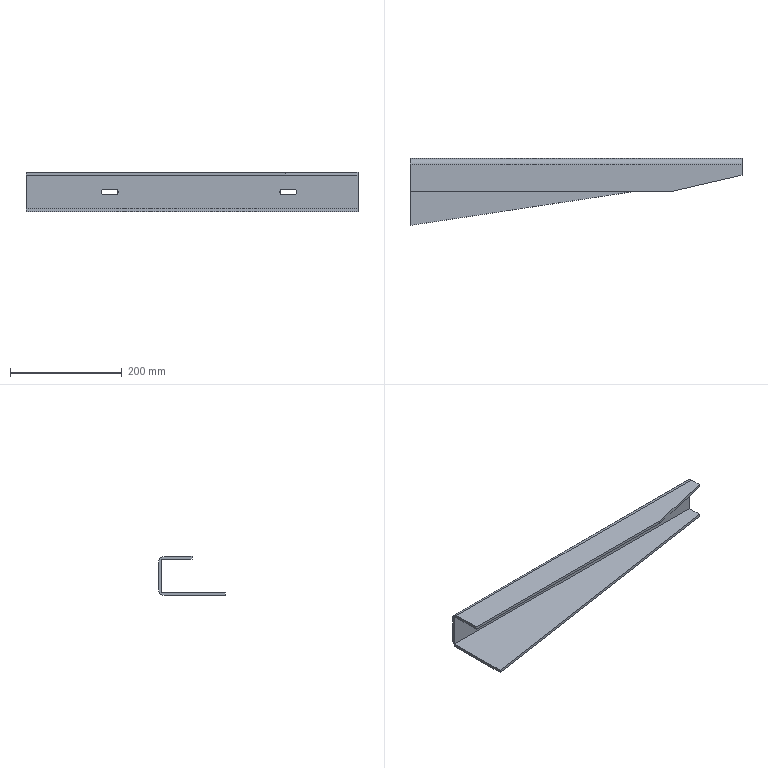Part | SolidWorks | features ICE 3, Fillet 2, Extrusion 1, Shell 1 | 1 solid | 21 faces | box 595 x 120 x 70 mm | volume 542052 mm3 | plane 15 | cylinder 6 | commonest cylinder face diameters 10 x4 20 x2
STEP:
#1=CARTESIAN_POINT('',(160.,70.,40.));
#2=VERTEX_POINT('',#1);
#3=CARTESIAN_POINT('',(140.,70.,40.));
#4=VERTEX_POINT('',#3);
#5=CARTESIAN_POINT('',(0.,70.,40.));
#6=DIRECTION('',(-1.,0.,0.));
#7=VECTOR('',#6,1000.);
#8=LINE('',#5,#7);
#9=EDGE_CURVE('',#2,#4,#8,.T.);
#10=ORIENTED_EDGE('',*,*,#9,.T.);
#11=CARTESIAN_POINT('',(140.,70.,30.));
#12=VERTEX_POINT('',#11);
#13=CARTESIAN_POINT('',(140.,70.,35.));
#14=DIRECTION('',(0.,1.,0.));
#15=DIRECTION('',(0.,0.,1.));
#16=AXIS2_PLACEMENT_3D('',#13,#14,#15);
#17=CIRCLE('',#16,5.);
#18=EDGE_CURVE('',#12,#4,#17,.T.);
#19=ORIENTED_EDGE('',*,*,#18,.F.);
#20=CARTESIAN_POINT('',(160.,70.,30.));
#21=VERTEX_POINT('',#20);
#22=CARTESIAN_POINT('',(0.,70.,30.));
#23=DIRECTION('',(1.,0.,0.));
#24=VECTOR('',#23,1000.);
#25=LINE('',#22,#24);
#26=EDGE_CURVE('',#12,#21,#25,.T.);
#27=ORIENTED_EDGE('',*,*,#26,.T.);
#28=CARTESIAN_POINT('',(160.,70.,35.));
#29=DIRECTION('',(0.,1.,0.));
#30=DIRECTION('',(0.,0.,1.));
#31=AXIS2_PLACEMENT_3D('',#28,#29,#30);
#32=CIRCLE('',#31,5.);
#33=EDGE_CURVE('',#2,#21,#32,.T.);
#34=ORIENTED_EDGE('',*,*,#33,.F.);
#35=EDGE_LOOP('',(#10,#19,#27,#34));
#36=FACE_BOUND('',#35,.T.);
#37=CARTESIAN_POINT('',(595.,70.,60.));
#38=VERTEX_POINT('',#37);
#39=CARTESIAN_POINT('',(595.,70.,10.));
#40=VERTEX_POINT('',#39);
#41=CARTESIAN_POINT('',(595.,70.,70.));
#42=DIRECTION('',(0.,0.,-1.));
#43=VECTOR('',#42,1000.);
#44=LINE('',#41,#43);
#45=EDGE_CURVE('',#38,#40,#44,.T.);
#46=ORIENTED_EDGE('',*,*,#45,.T.);
#47=CARTESIAN_POINT('',(0.,70.,10.));
#48=VERTEX_POINT('',#47);
#49=CARTESIAN_POINT('',(0.,70.,10.));
#50=DIRECTION('',(-1.,0.,0.));
#51=VECTOR('',#50,1000.);
#52=LINE('',#49,#51);
#53=EDGE_CURVE('',#40,#48,#52,.T.);
#54=ORIENTED_EDGE('',*,*,#53,.T.);
#55=CARTESIAN_POINT('',(0.,70.,60.));
#56=VERTEX_POINT('',#55);
#57=CARTESIAN_POINT('',(0.,70.,70.));
#58=DIRECTION('',(0.,0.,-1.));
#59=VECTOR('',#58,1000.);
#60=LINE('',#57,#59);
#61=EDGE_CURVE('',#56,#48,#60,.T.);
#62=ORIENTED_EDGE('',*,*,#61,.F.);
#63=CARTESIAN_POINT('',(570.,70.,60.));
#64=DIRECTION('',(1.,0.,0.));
#65=VECTOR('',#64,1000.);
#66=LINE('',#63,#65);
#67=EDGE_CURVE('',#56,#38,#66,.T.);
#68=ORIENTED_EDGE('',*,*,#67,.T.);
#69=EDGE_LOOP('',(#46,#54,#62,#68));
#70=FACE_OUTER_BOUND('',#69,.T.);
#71=CARTESIAN_POINT('',(460.,70.,30.));
#72=VERTEX_POINT('',#71);
#73=CARTESIAN_POINT('',(480.,70.,30.));
#74=VERTEX_POINT('',#73);
#75=CARTESIAN_POINT('',(0.,70.,30.));
#76=DIRECTION('',(1.,0.,0.));
#77=VECTOR('',#76,1000.);
#78=LINE('',#75,#77);
#79=EDGE_CURVE('',#72,#74,#78,.T.);
#80=ORIENTED_EDGE('',*,*,#79,.T.);
#81=CARTESIAN_POINT('',(480.,70.,40.));
#82=VERTEX_POINT('',#81);
#83=CARTESIAN_POINT('',(480.,70.,35.));
#84=DIRECTION('',(0.,1.,0.));
#85=DIRECTION('',(0.,0.,1.));
#86=AXIS2_PLACEMENT_3D('',#83,#84,#85);
#87=CIRCLE('',#86,5.);
#88=EDGE_CURVE('',#82,#74,#87,.T.);
#89=ORIENTED_EDGE('',*,*,#88,.F.);
#90=CARTESIAN_POINT('',(460.,70.,40.));
#91=VERTEX_POINT('',#90);
#92=CARTESIAN_POINT('',(0.,70.,40.));
#93=DIRECTION('',(-1.,0.,0.));
#94=VECTOR('',#93,1000.);
#95=LINE('',#92,#94);
#96=EDGE_CURVE('',#82,#91,#95,.T.);
#97=ORIENTED_EDGE('',*,*,#96,.T.);
#98=CARTESIAN_POINT('',(460.,70.,35.));
#99=DIRECTION('',(0.,1.,0.));
#100=DIRECTION('',(0.,0.,1.));
#101=AXIS2_PLACEMENT_3D('',#98,#99,#100);
#102=CIRCLE('',#101,5.);
#103=EDGE_CURVE('',#72,#91,#102,.T.);
#104=ORIENTED_EDGE('',*,*,#103,.F.);
#105=EDGE_LOOP('',(#80,#89,#97,#104));
#106=FACE_BOUND('',#105,.T.);
#107=CARTESIAN_POINT('',(570.,70.,70.));
#108=DIRECTION('',(0.,-1.,0.));
#109=DIRECTION('',(0.,0.,-1.));
#110=AXIS2_PLACEMENT_3D('',#107,#108,#109);
#111=PLANE('',#110);
#112=ADVANCED_FACE('',(#36,#70,#106),#111,.F.);
#113=CARTESIAN_POINT('',(140.,65.,30.));
#114=VERTEX_POINT('',#113);
#115=CARTESIAN_POINT('',(140.,65.,40.));
#116=VERTEX_POINT('',#115);
#117=CARTESIAN_POINT('',(140.,65.,35.));
#118=DIRECTION('',(0.,1.,0.));
#119=DIRECTION('',(0.,0.,1.));
#120=AXIS2_PLACEMENT_3D('',#117,#118,#119);
#121=CIRCLE('',#120,5.);
#122=EDGE_CURVE('',#114,#116,#121,.T.);
#123=ORIENTED_EDGE('',*,*,#122,.T.);
#124=CARTESIAN_POINT('',(160.,65.,40.));
#125=VERTEX_POINT('',#124);
#126=CARTESIAN_POINT('',(0.,65.,40.));
#127=DIRECTION('',(-1.,0.,0.));
#128=VECTOR('',#127,1000.);
#129=LINE('',#126,#128);
#130=EDGE_CURVE('',#125,#116,#129,.T.);
#131=ORIENTED_EDGE('',*,*,#130,.F.);
#132=CARTESIAN_POINT('',(160.,65.,30.));
#133=VERTEX_POINT('',#132);
#134=CARTESIAN_POINT('',(160.,65.,35.));
#135=DIRECTION('',(0.,1.,0.));
#136=DIRECTION('',(0.,0.,1.));
#137=AXIS2_PLACEMENT_3D('',#134,#135,#136);
#138=CIRCLE('',#137,5.);
#139=EDGE_CURVE('',#125,#133,#138,.T.);
#140=ORIENTED_EDGE('',*,*,#139,.T.);
#141=CARTESIAN_POINT('',(0.,65.,30.));
#142=DIRECTION('',(1.,0.,0.));
#143=VECTOR('',#142,1000.);
#144=LINE('',#141,#143);
#145=EDGE_CURVE('',#114,#133,#144,.T.);
#146=ORIENTED_EDGE('',*,*,#145,.F.);
#147=EDGE_LOOP('',(#123,#131,#140,#146));
#148=FACE_BOUND('',#147,.T.);
#149=CARTESIAN_POINT('',(595.,65.,5.));
#150=VERTEX_POINT('',#149);
#151=CARTESIAN_POINT('',(0.,65.,5.));
#152=VERTEX_POINT('',#151);
#153=CARTESIAN_POINT('',(0.,65.,5.));
#154=DIRECTION('',(-1.,0.,0.));
#155=VECTOR('',#154,1000.);
#156=LINE('',#153,#155);
#157=EDGE_CURVE('',#150,#152,#156,.T.);
#158=ORIENTED_EDGE('',*,*,#157,.F.);
#159=CARTESIAN_POINT('',(595.,65.,65.));
#160=VERTEX_POINT('',#159);
#161=CARTESIAN_POINT('',(595.,65.,70.));
#162=DIRECTION('',(0.,0.,-1.));
#163=VECTOR('',#162,1000.);
#164=LINE('',#161,#163);
#165=EDGE_CURVE('',#160,#150,#164,.T.);
#166=ORIENTED_EDGE('',*,*,#165,.F.);
#167=CARTESIAN_POINT('',(0.,65.,65.));
#168=VERTEX_POINT('',#167);
#169=CARTESIAN_POINT('',(0.,65.,65.));
#170=DIRECTION('',(-1.,0.,0.));
#171=VECTOR('',#170,1000.);
#172=LINE('',#169,#171);
#173=EDGE_CURVE('',#160,#168,#172,.T.);
#174=ORIENTED_EDGE('',*,*,#173,.T.);
#175=CARTESIAN_POINT('',(0.,65.,70.));
#176=DIRECTION('',(0.,0.,-1.));
#177=VECTOR('',#176,1000.);
#178=LINE('',#175,#177);
#179=EDGE_CURVE('',#168,#152,#178,.T.);
#180=ORIENTED_EDGE('',*,*,#179,.T.);
#181=EDGE_LOOP('',(#158,#166,#174,#180));
#182=FACE_OUTER_BOUND('',#181,.T.);
#183=CARTESIAN_POINT('',(480.,65.,40.));
#184=VERTEX_POINT('',#183);
#185=CARTESIAN_POINT('',(480.,65.,30.));
#186=VERTEX_POINT('',#185);
#187=CARTESIAN_POINT('',(480.,65.,35.));
#188=DIRECTION('',(0.,1.,0.));
#189=DIRECTION('',(0.,0.,1.));
#190=AXIS2_PLACEMENT_3D('',#187,#188,#189);
#191=CIRCLE('',#190,5.);
#192=EDGE_CURVE('',#184,#186,#191,.T.);
#193=ORIENTED_EDGE('',*,*,#192,.T.);
#194=CARTESIAN_POINT('',(460.,65.,30.));
#195=VERTEX_POINT('',#194);
#196=CARTESIAN_POINT('',(0.,65.,30.));
#197=DIRECTION('',(1.,0.,0.));
#198=VECTOR('',#197,1000.);
#199=LINE('',#196,#198);
#200=EDGE_CURVE('',#195,#186,#199,.T.);
#201=ORIENTED_EDGE('',*,*,#200,.F.);
#202=CARTESIAN_POINT('',(460.,65.,40.));
#203=VERTEX_POINT('',#202);
#204=CARTESIAN_POINT('',(460.,65.,35.));
#205=DIRECTION('',(0.,1.,0.));
#206=DIRECTION('',(0.,0.,1.));
#207=AXIS2_PLACEMENT_3D('',#204,#205,#206);
#208=CIRCLE('',#207,5.);
#209=EDGE_CURVE('',#195,#203,#208,.T.);
#210=ORIENTED_EDGE('',*,*,#209,.T.);
#211=CARTESIAN_POINT('',(0.,65.,40.));
#212=DIRECTION('',(-1.,0.,0.));
#213=VECTOR('',#212,1000.);
#214=LINE('',#211,#213);
#215=EDGE_CURVE('',#184,#203,#214,.T.);
#216=ORIENTED_EDGE('',*,*,#215,.F.);
#217=EDGE_LOOP('',(#193,#201,#210,#216));
#218=FACE_BOUND('',#217,.T.);
#219=CARTESIAN_POINT('',(570.,65.,70.));
#220=DIRECTION('',(0.,-1.,0.));
#221=DIRECTION('',(0.,0.,-1.));
#222=AXIS2_PLACEMENT_3D('',#219,#220,#221);
#223=PLANE('',#222);
#224=ADVANCED_FACE('',(#148,#182,#218),#223,.T.);
#225=CARTESIAN_POINT('',(0.,60.,0.));
#226=VERTEX_POINT('',#225);
#227=CARTESIAN_POINT('',(595.,60.,0.));
#228=VERTEX_POINT('',#227);
#229=CARTESIAN_POINT('',(0.,60.,0.));
#230=DIRECTION('',(1.,0.,0.));
#231=VECTOR('',#230,1000.);
#232=LINE('',#229,#231);
#233=EDGE_CURVE('',#226,#228,#232,.T.);
#234=ORIENTED_EDGE('',*,*,#233,.F.);
#235=CARTESIAN_POINT('',(0.,60.,10.));
#236=DIRECTION('',(-1.,0.,0.));
#237=DIRECTION('',(0.,1.,0.));
#238=AXIS2_PLACEMENT_3D('',#235,#236,#237);
#239=CIRCLE('',#238,10.);
#240=EDGE_CURVE('',#48,#226,#239,.T.);
#241=ORIENTED_EDGE('',*,*,#240,.F.);
#242=ORIENTED_EDGE('',*,*,#53,.F.);
#243=CARTESIAN_POINT('',(595.,60.,10.));
#244=DIRECTION('',(1.,0.,0.));
#245=DIRECTION('',(0.,0.,1.));
#246=AXIS2_PLACEMENT_3D('',#243,#244,#245);
#247=CIRCLE('',#246,10.);
#248=EDGE_CURVE('',#228,#40,#247,.T.);
#249=ORIENTED_EDGE('',*,*,#248,.F.);
#250=EDGE_LOOP('',(#234,#241,#242,#249));
#251=FACE_OUTER_BOUND('',#250,.T.);
#252=CARTESIAN_POINT('',(0.,60.,10.));
#253=DIRECTION('',(-1.,0.,0.));
#254=DIRECTION('',(0.,0.,1.));
#255=AXIS2_PLACEMENT_3D('',#252,#253,#254);
#256=CYLINDRICAL_SURFACE('',#255,10.);
#257=ADVANCED_FACE('',(#251),#256,.T.);
#258=ORIENTED_EDGE('',*,*,#67,.F.);
#259=CARTESIAN_POINT('',(0.,60.,70.));
#260=VERTEX_POINT('',#259);
#261=CARTESIAN_POINT('',(0.,60.,60.));
#262=DIRECTION('',(-1.,0.,0.));
#263=DIRECTION('',(0.,1.,0.));
#264=AXIS2_PLACEMENT_3D('',#261,#262,#263);
#265=CIRCLE('',#264,10.);
#266=EDGE_CURVE('',#260,#56,#265,.T.);
#267=ORIENTED_EDGE('',*,*,#266,.F.);
#268=CARTESIAN_POINT('',(595.,60.,70.));
#269=VERTEX_POINT('',#268);
#270=CARTESIAN_POINT('',(0.,60.,70.));
#271=DIRECTION('',(-1.,0.,0.));
#272=VECTOR('',#271,1000.);
#273=LINE('',#270,#272);
#274=EDGE_CURVE('',#269,#260,#273,.T.);
#275=ORIENTED_EDGE('',*,*,#274,.F.);
#276=CARTESIAN_POINT('',(595.,60.,60.));
#277=DIRECTION('',(1.,0.,0.));
#278=DIRECTION('',(0.,0.,1.));
#279=AXIS2_PLACEMENT_3D('',#276,#277,#278);
#280=CIRCLE('',#279,10.);
#281=EDGE_CURVE('',#38,#269,#280,.T.);
#282=ORIENTED_EDGE('',*,*,#281,.F.);
#283=EDGE_LOOP('',(#258,#267,#275,#282));
#284=FACE_OUTER_BOUND('',#283,.T.);
#285=CARTESIAN_POINT('',(570.,60.,60.));
#286=DIRECTION('',(1.,0.,0.));
#287=DIRECTION('',(0.,0.,-1.));
#288=AXIS2_PLACEMENT_3D('',#285,#286,#287);
#289=CYLINDRICAL_SURFACE('',#288,10.);
#290=ADVANCED_FACE('',(#284),#289,.T.);
#291=ORIENTED_EDGE('',*,*,#61,.T.);
#292=ORIENTED_EDGE('',*,*,#240,.T.);
#293=CARTESIAN_POINT('',(0.,-50.,0.));
#294=VERTEX_POINT('',#293);
#295=CARTESIAN_POINT('',(0.,70.,0.));
#296=DIRECTION('',(0.,-1.,0.));
#297=VECTOR('',#296,1000.);
#298=LINE('',#295,#297);
#299=EDGE_CURVE('',#226,#294,#298,.T.);
#300=ORIENTED_EDGE('',*,*,#299,.T.);
#301=CARTESIAN_POINT('',(0.,-50.,5.));
#302=VERTEX_POINT('',#301);
#303=CARTESIAN_POINT('',(0.,-50.,70.));
#304=DIRECTION('',(0.,0.,-1.));
#305=VECTOR('',#304,1000.);
#306=LINE('',#303,#305);
#307=EDGE_CURVE('',#302,#294,#306,.T.);
#308=ORIENTED_EDGE('',*,*,#307,.F.);
#309=CARTESIAN_POINT('',(0.,0.,5.));
#310=DIRECTION('',(0.,-1.,0.));
#311=VECTOR('',#310,1000.);
#312=LINE('',#309,#311);
#313=EDGE_CURVE('',#152,#302,#312,.T.);
#314=ORIENTED_EDGE('',*,*,#313,.F.);
#315=ORIENTED_EDGE('',*,*,#179,.F.);
#316=CARTESIAN_POINT('',(0.,10.,65.));
#317=VERTEX_POINT('',#316);
#318=CARTESIAN_POINT('',(0.,0.,65.));
#319=DIRECTION('',(0.,-1.,0.));
#320=VECTOR('',#319,1000.);
#321=LINE('',#318,#320);
#322=EDGE_CURVE('',#168,#317,#321,.T.);
#323=ORIENTED_EDGE('',*,*,#322,.T.);
#324=CARTESIAN_POINT('',(0.,10.,70.));
#325=VERTEX_POINT('',#324);
#326=CARTESIAN_POINT('',(0.,10.,65.));
#327=DIRECTION('',(0.,0.,1.));
#328=VECTOR('',#327,1000.);
#329=LINE('',#326,#328);
#330=EDGE_CURVE('',#317,#325,#329,.T.);
#331=ORIENTED_EDGE('',*,*,#330,.T.);
#332=CARTESIAN_POINT('',(0.,70.,70.));
#333=DIRECTION('',(0.,-1.,0.));
#334=VECTOR('',#333,1000.);
#335=LINE('',#332,#334);
#336=EDGE_CURVE('',#260,#325,#335,.T.);
#337=ORIENTED_EDGE('',*,*,#336,.F.);
#338=ORIENTED_EDGE('',*,*,#266,.T.);
#339=EDGE_LOOP('',(#291,#292,#300,#308,#314,#315,#323,#331,#337,#338));
#340=FACE_OUTER_BOUND('',#339,.T.);
#341=CARTESIAN_POINT('',(0.,70.,70.));
#342=DIRECTION('',(1.,0.,0.));
#343=DIRECTION('',(0.,1.,0.));
#344=AXIS2_PLACEMENT_3D('',#341,#342,#343);
#345=PLANE('',#344);
#346=ADVANCED_FACE('',(#340),#345,.F.);
#347=CARTESIAN_POINT('',(595.,40.,5.));
#348=VERTEX_POINT('',#347);
#349=CARTESIAN_POINT('',(7.394,-48.882,5.));
#350=DIRECTION('',(0.9888,0.1496,0.));
#351=VECTOR('',#350,1000.);
#352=LINE('',#349,#351);
#353=EDGE_CURVE('',#302,#348,#352,.T.);
#354=ORIENTED_EDGE('',*,*,#353,.F.);
#355=ORIENTED_EDGE('',*,*,#307,.T.);
#356=CARTESIAN_POINT('',(595.,40.,0.));
#357=VERTEX_POINT('',#356);
#358=CARTESIAN_POINT('',(595.,40.,0.));
#359=DIRECTION('',(0.9888,0.1496,0.));
#360=VECTOR('',#359,1000.);
#361=LINE('',#358,#360);
#362=EDGE_CURVE('',#294,#357,#361,.T.);
#363=ORIENTED_EDGE('',*,*,#362,.T.);
#364=CARTESIAN_POINT('',(595.,40.,70.));
#365=DIRECTION('',(0.,0.,-1.));
#366=VECTOR('',#365,1000.);
#367=LINE('',#364,#366);
#368=EDGE_CURVE('',#348,#357,#367,.T.);
#369=ORIENTED_EDGE('',*,*,#368,.F.);
#370=EDGE_LOOP('',(#354,#355,#363,#369));
#371=FACE_OUTER_BOUND('',#370,.T.);
#372=CARTESIAN_POINT('',(595.,40.,70.));
#373=DIRECTION('',(-0.1496,0.9888,0.));
#374=DIRECTION('',(-0.9888,-0.1496,0.));
#375=AXIS2_PLACEMENT_3D('',#372,#373,#374);
#376=PLANE('',#375);
#377=ADVANCED_FACE('',(#371),#376,.F.);
#378=CARTESIAN_POINT('',(595.,70.,0.));
#379=DIRECTION('',(0.,1.,0.));
#380=VECTOR('',#379,1000.);
#381=LINE('',#378,#380);
#382=EDGE_CURVE('',#357,#228,#381,.T.);
#383=ORIENTED_EDGE('',*,*,#382,.T.);
#384=ORIENTED_EDGE('',*,*,#248,.T.);
#385=ORIENTED_EDGE('',*,*,#45,.F.);
#386=ORIENTED_EDGE('',*,*,#281,.T.);
#387=CARTESIAN_POINT('',(595.,40.,70.));
#388=VERTEX_POINT('',#387);
#389=CARTESIAN_POINT('',(595.,70.,70.));
#390=DIRECTION('',(0.,1.,0.));
#391=VECTOR('',#390,1000.);
#392=LINE('',#389,#391);
#393=EDGE_CURVE('',#388,#269,#392,.T.);
#394=ORIENTED_EDGE('',*,*,#393,.F.);
#395=CARTESIAN_POINT('',(595.,40.,65.));
#396=VERTEX_POINT('',#395);
#397=CARTESIAN_POINT('',(595.,40.,70.));
#398=DIRECTION('',(0.,0.,-1.));
#399=VECTOR('',#398,1000.);
#400=LINE('',#397,#399);
#401=EDGE_CURVE('',#388,#396,#400,.T.);
#402=ORIENTED_EDGE('',*,*,#401,.T.);
#403=CARTESIAN_POINT('',(595.,0.,65.));
#404=DIRECTION('',(0.,1.,0.));
#405=VECTOR('',#404,1000.);
#406=LINE('',#403,#405);
#407=EDGE_CURVE('',#396,#160,#406,.T.);
#408=ORIENTED_EDGE('',*,*,#407,.T.);
#409=ORIENTED_EDGE('',*,*,#165,.T.);
#410=CARTESIAN_POINT('',(595.,0.,5.));
#411=DIRECTION('',(0.,1.,0.));
#412=VECTOR('',#411,1000.);
#413=LINE('',#410,#412);
#414=EDGE_CURVE('',#348,#150,#413,.T.);
#415=ORIENTED_EDGE('',*,*,#414,.F.);
#416=ORIENTED_EDGE('',*,*,#368,.T.);
#417=EDGE_LOOP('',(#383,#384,#385,#386,#394,#402,#408,#409,#415,#416));
#418=FACE_OUTER_BOUND('',#417,.T.);
#419=CARTESIAN_POINT('',(595.,70.,70.));
#420=DIRECTION('',(-1.,0.,0.));
#421=DIRECTION('',(0.,0.,1.));
#422=AXIS2_PLACEMENT_3D('',#419,#420,#421);
#423=PLANE('',#422);
#424=ADVANCED_FACE('',(#418),#423,.F.);
#425=ORIENTED_EDGE('',*,*,#393,.T.);
#426=ORIENTED_EDGE('',*,*,#274,.T.);
#427=ORIENTED_EDGE('',*,*,#336,.T.);
#428=CARTESIAN_POINT('',(465.,10.,70.));
#429=VERTEX_POINT('',#428);
#430=CARTESIAN_POINT('',(0.,10.,70.));
#431=DIRECTION('',(1.,0.,0.));
#432=VECTOR('',#431,1000.);
#433=LINE('',#430,#432);
#434=EDGE_CURVE('',#325,#429,#433,.T.);
#435=ORIENTED_EDGE('',*,*,#434,.T.);
#436=CARTESIAN_POINT('',(21.32,-92.388,70.));
#437=DIRECTION('',(0.9744,0.2249,0.));
#438=VECTOR('',#437,1000.);
#439=LINE('',#436,#438);
#440=EDGE_CURVE('',#429,#388,#439,.T.);
#441=ORIENTED_EDGE('',*,*,#440,.T.);
#442=EDGE_LOOP('',(#425,#426,#427,#435,#441));
#443=FACE_OUTER_BOUND('',#442,.T.);
#444=CARTESIAN_POINT('',(0.,0.,70.));
#445=DIRECTION('',(0.,0.,-1.));
#446=DIRECTION('',(-1.,0.,0.));
#447=AXIS2_PLACEMENT_3D('',#444,#445,#446);
#448=PLANE('',#447);
#449=ADVANCED_FACE('',(#443),#448,.F.);
#450=ORIENTED_EDGE('',*,*,#299,.F.);
#451=ORIENTED_EDGE('',*,*,#233,.T.);
#452=ORIENTED_EDGE('',*,*,#382,.F.);
#453=ORIENTED_EDGE('',*,*,#362,.F.);
#454=EDGE_LOOP('',(#450,#451,#452,#453));
#455=FACE_OUTER_BOUND('',#454,.T.);
#456=CARTESIAN_POINT('',(0.,0.,0.));
#457=DIRECTION('',(0.,0.,-1.));
#458=DIRECTION('',(-1.,0.,0.));
#459=AXIS2_PLACEMENT_3D('',#456,#457,#458);
#460=PLANE('',#459);
#461=ADVANCED_FACE('',(#455),#460,.T.);
#462=CARTESIAN_POINT('',(465.,10.,65.));
#463=VERTEX_POINT('',#462);
#464=CARTESIAN_POINT('',(0.,10.,65.));
#465=DIRECTION('',(1.,0.,0.));
#466=VECTOR('',#465,1000.);
#467=LINE('',#464,#466);
#468=EDGE_CURVE('',#317,#463,#467,.T.);
#469=ORIENTED_EDGE('',*,*,#468,.F.);
#470=ORIENTED_EDGE('',*,*,#322,.F.);
#471=ORIENTED_EDGE('',*,*,#173,.F.);
#472=ORIENTED_EDGE('',*,*,#407,.F.);
#473=CARTESIAN_POINT('',(21.32,-92.388,65.));
#474=DIRECTION('',(0.9744,0.2249,0.));
#475=VECTOR('',#474,1000.);
#476=LINE('',#473,#475);
#477=EDGE_CURVE('',#463,#396,#476,.T.);
#478=ORIENTED_EDGE('',*,*,#477,.F.);
#479=EDGE_LOOP('',(#469,#470,#471,#472,#478));
#480=FACE_OUTER_BOUND('',#479,.T.);
#481=CARTESIAN_POINT('',(0.,0.,65.));
#482=DIRECTION('',(0.,0.,-1.));
#483=DIRECTION('',(-1.,0.,0.));
#484=AXIS2_PLACEMENT_3D('',#481,#482,#483);
#485=PLANE('',#484);
#486=ADVANCED_FACE('',(#480),#485,.T.);
#487=ORIENTED_EDGE('',*,*,#313,.T.);
#488=ORIENTED_EDGE('',*,*,#353,.T.);
#489=ORIENTED_EDGE('',*,*,#414,.T.);
#490=ORIENTED_EDGE('',*,*,#157,.T.);
#491=EDGE_LOOP('',(#487,#488,#489,#490));
#492=FACE_OUTER_BOUND('',#491,.T.);
#493=CARTESIAN_POINT('',(0.,0.,5.));
#494=DIRECTION('',(0.,0.,-1.));
#495=DIRECTION('',(-1.,0.,0.));
#496=AXIS2_PLACEMENT_3D('',#493,#494,#495);
#497=PLANE('',#496);
#498=ADVANCED_FACE('',(#492),#497,.F.);
#499=ORIENTED_EDGE('',*,*,#434,.F.);
#500=ORIENTED_EDGE('',*,*,#330,.F.);
#501=ORIENTED_EDGE('',*,*,#468,.T.);
#502=CARTESIAN_POINT('',(465.,10.,65.));
#503=DIRECTION('',(0.,0.,1.));
#504=VECTOR('',#503,1000.);
#505=LINE('',#502,#504);
#506=EDGE_CURVE('',#463,#429,#505,.T.);
#507=ORIENTED_EDGE('',*,*,#506,.T.);
#508=EDGE_LOOP('',(#499,#500,#501,#507));
#509=FACE_OUTER_BOUND('',#508,.T.);
#510=CARTESIAN_POINT('',(0.,10.,65.));
#511=DIRECTION('',(0.,-1.,0.));
#512=DIRECTION('',(0.,0.,-1.));
#513=AXIS2_PLACEMENT_3D('',#510,#511,#512);
#514=PLANE('',#513);
#515=ADVANCED_FACE('',(#509),#514,.T.);
#516=ORIENTED_EDGE('',*,*,#440,.F.);
#517=ORIENTED_EDGE('',*,*,#506,.F.);
#518=ORIENTED_EDGE('',*,*,#477,.T.);
#519=ORIENTED_EDGE('',*,*,#401,.F.);
#520=EDGE_LOOP('',(#516,#517,#518,#519));
#521=FACE_OUTER_BOUND('',#520,.T.);
#522=CARTESIAN_POINT('',(21.32,-92.388,65.));
#523=DIRECTION('',(0.2249,-0.9744,0.));
#524=DIRECTION('',(0.9744,0.2249,0.));
#525=AXIS2_PLACEMENT_3D('',#522,#523,#524);
#526=PLANE('',#525);
#527=ADVANCED_FACE('',(#521),#526,.T.);
#528=ORIENTED_EDGE('',*,*,#9,.F.);
#529=CARTESIAN_POINT('',(160.,65.,40.));
#530=DIRECTION('',(0.,1.,0.));
#531=VECTOR('',#530,1000.);
#532=LINE('',#529,#531);
#533=EDGE_CURVE('',#125,#2,#532,.T.);
#534=ORIENTED_EDGE('',*,*,#533,.F.);
#535=ORIENTED_EDGE('',*,*,#130,.T.);
#536=CARTESIAN_POINT('',(140.,65.,40.));
#537=DIRECTION('',(0.,1.,0.));
#538=VECTOR('',#537,1000.);
#539=LINE('',#536,#538);
#540=EDGE_CURVE('',#116,#4,#539,.T.);
#541=ORIENTED_EDGE('',*,*,#540,.T.);
#542=EDGE_LOOP('',(#528,#534,#535,#541));
#543=FACE_OUTER_BOUND('',#542,.T.);
#544=CARTESIAN_POINT('',(0.,65.,40.));
#545=DIRECTION('',(0.,0.,-1.));
#546=DIRECTION('',(-1.,0.,0.));
#547=AXIS2_PLACEMENT_3D('',#544,#545,#546);
#548=PLANE('',#547);
#549=ADVANCED_FACE('',(#543),#548,.T.);
#550=ORIENTED_EDGE('',*,*,#18,.T.);
#551=ORIENTED_EDGE('',*,*,#540,.F.);
#552=ORIENTED_EDGE('',*,*,#122,.F.);
#553=CARTESIAN_POINT('',(140.,65.,30.));
#554=DIRECTION('',(0.,1.,0.));
#555=VECTOR('',#554,1000.);
#556=LINE('',#553,#555);
#557=EDGE_CURVE('',#114,#12,#556,.T.);
#558=ORIENTED_EDGE('',*,*,#557,.T.);
#559=EDGE_LOOP('',(#550,#551,#552,#558));
#560=FACE_OUTER_BOUND('',#559,.T.);
#561=CARTESIAN_POINT('',(140.,65.,35.));
#562=DIRECTION('',(0.,1.,0.));
#563=DIRECTION('',(0.,0.,1.));
#564=AXIS2_PLACEMENT_3D('',#561,#562,#563);
#565=CYLINDRICAL_SURFACE('',#564,5.);
#566=ADVANCED_FACE('',(#560),#565,.F.);
#567=ORIENTED_EDGE('',*,*,#26,.F.);
#568=ORIENTED_EDGE('',*,*,#557,.F.);
#569=ORIENTED_EDGE('',*,*,#145,.T.);
#570=CARTESIAN_POINT('',(160.,65.,30.));
#571=DIRECTION('',(0.,1.,0.));
#572=VECTOR('',#571,1000.);
#573=LINE('',#570,#572);
#574=EDGE_CURVE('',#133,#21,#573,.T.);
#575=ORIENTED_EDGE('',*,*,#574,.T.);
#576=EDGE_LOOP('',(#567,#568,#569,#575));
#577=FACE_OUTER_BOUND('',#576,.T.);
#578=CARTESIAN_POINT('',(0.,65.,30.));
#579=DIRECTION('',(0.,0.,1.));
#580=DIRECTION('',(1.,0.,0.));
#581=AXIS2_PLACEMENT_3D('',#578,#579,#580);
#582=PLANE('',#581);
#583=ADVANCED_FACE('',(#577),#582,.T.);
#584=ORIENTED_EDGE('',*,*,#33,.T.);
#585=ORIENTED_EDGE('',*,*,#574,.F.);
#586=ORIENTED_EDGE('',*,*,#139,.F.);
#587=ORIENTED_EDGE('',*,*,#533,.T.);
#588=EDGE_LOOP('',(#584,#585,#586,#587));
#589=FACE_OUTER_BOUND('',#588,.T.);
#590=CARTESIAN_POINT('',(160.,65.,35.));
#591=DIRECTION('',(0.,1.,0.));
#592=DIRECTION('',(0.,0.,1.));
#593=AXIS2_PLACEMENT_3D('',#590,#591,#592);
#594=CYLINDRICAL_SURFACE('',#593,5.);
#595=ADVANCED_FACE('',(#589),#594,.F.);
#596=ORIENTED_EDGE('',*,*,#79,.F.);
#597=CARTESIAN_POINT('',(460.,65.,30.));
#598=DIRECTION('',(0.,1.,0.));
#599=VECTOR('',#598,1000.);
#600=LINE('',#597,#599);
#601=EDGE_CURVE('',#195,#72,#600,.T.);
#602=ORIENTED_EDGE('',*,*,#601,.F.);
#603=ORIENTED_EDGE('',*,*,#200,.T.);
#604=CARTESIAN_POINT('',(480.,65.,30.));
#605=DIRECTION('',(0.,1.,0.));
#606=VECTOR('',#605,1000.);
#607=LINE('',#604,#606);
#608=EDGE_CURVE('',#186,#74,#607,.T.);
#609=ORIENTED_EDGE('',*,*,#608,.T.);
#610=EDGE_LOOP('',(#596,#602,#603,#609));
#611=FACE_OUTER_BOUND('',#610,.T.);
#612=CARTESIAN_POINT('',(0.,65.,30.));
#613=DIRECTION('',(0.,0.,1.));
#614=DIRECTION('',(1.,0.,0.));
#615=AXIS2_PLACEMENT_3D('',#612,#613,#614);
#616=PLANE('',#615);
#617=ADVANCED_FACE('',(#611),#616,.T.);
#618=ORIENTED_EDGE('',*,*,#88,.T.);
#619=ORIENTED_EDGE('',*,*,#608,.F.);
#620=ORIENTED_EDGE('',*,*,#192,.F.);
#621=CARTESIAN_POINT('',(480.,65.,40.));
#622=DIRECTION('',(0.,1.,0.));
#623=VECTOR('',#622,1000.);
#624=LINE('',#621,#623);
#625=EDGE_CURVE('',#184,#82,#624,.T.);
#626=ORIENTED_EDGE('',*,*,#625,.T.);
#627=EDGE_LOOP('',(#618,#619,#620,#626));
#628=FACE_OUTER_BOUND('',#627,.T.);
#629=CARTESIAN_POINT('',(480.,65.,35.));
#630=DIRECTION('',(0.,1.,0.));
#631=DIRECTION('',(0.,0.,1.));
#632=AXIS2_PLACEMENT_3D('',#629,#630,#631);
#633=CYLINDRICAL_SURFACE('',#632,5.);
#634=ADVANCED_FACE('',(#628),#633,.F.);
#635=ORIENTED_EDGE('',*,*,#96,.F.);
#636=ORIENTED_EDGE('',*,*,#625,.F.);
#637=ORIENTED_EDGE('',*,*,#215,.T.);
#638=CARTESIAN_POINT('',(460.,65.,40.));
#639=DIRECTION('',(0.,1.,0.));
#640=VECTOR('',#639,1000.);
#641=LINE('',#638,#640);
#642=EDGE_CURVE('',#203,#91,#641,.T.);
#643=ORIENTED_EDGE('',*,*,#642,.T.);
#644=EDGE_LOOP('',(#635,#636,#637,#643));
#645=FACE_OUTER_BOUND('',#644,.T.);
#646=CARTESIAN_POINT('',(0.,65.,40.));
#647=DIRECTION('',(0.,0.,-1.));
#648=DIRECTION('',(-1.,0.,0.));
#649=AXIS2_PLACEMENT_3D('',#646,#647,#648);
#650=PLANE('',#649);
#651=ADVANCED_FACE('',(#645),#650,.T.);
#652=ORIENTED_EDGE('',*,*,#103,.T.);
#653=ORIENTED_EDGE('',*,*,#642,.F.);
#654=ORIENTED_EDGE('',*,*,#209,.F.);
#655=ORIENTED_EDGE('',*,*,#601,.T.);
#656=EDGE_LOOP('',(#652,#653,#654,#655));
#657=FACE_OUTER_BOUND('',#656,.T.);
#658=CARTESIAN_POINT('',(460.,65.,35.));
#659=DIRECTION('',(0.,1.,0.));
#660=DIRECTION('',(0.,0.,1.));
#661=AXIS2_PLACEMENT_3D('',#658,#659,#660);
#662=CYLINDRICAL_SURFACE('',#661,5.);
#663=ADVANCED_FACE('',(#657),#662,.F.);
#664=CLOSED_SHELL('',(#112,#224,#257,#290,#346,#377,#424,#449,#461,#486,#498,#515,#527,#549,#566,#583,#595,#617,#634,#651,#663));
#665=MANIFOLD_SOLID_BREP('',#664);
#666=CARTESIAN_POINT('',(0.,0.,0.));
#667=DIRECTION('',(0.,0.,1.));
#668=DIRECTION('',(1.,0.,0.));
#669=AXIS2_PLACEMENT_3D('',#666,#667,#668);
#670=(LENGTH_UNIT()NAMED_UNIT(*)SI_UNIT(.MILLI.,.METRE.));
#671=UNCERTAINTY_MEASURE_WITH_UNIT(LENGTH_MEASURE(0.00001),#670,'','');
#672=(NAMED_UNIT(*)PLANE_ANGLE_UNIT()SI_UNIT($,.RADIAN.));
#673=(NAMED_UNIT(*)SI_UNIT($,.STERADIAN.)SOLID_ANGLE_UNIT());
#674=(GEOMETRIC_REPRESENTATION_CONTEXT(3)GLOBAL_UNCERTAINTY_ASSIGNED_CONTEXT((#671))GLOBAL_UNIT_ASSIGNED_CONTEXT((#670,#672,#673))REPRESENTATION_CONTEXT('',''));
#675=ADVANCED_BREP_SHAPE_REPRESENTATION('',(#665,#669),#674);